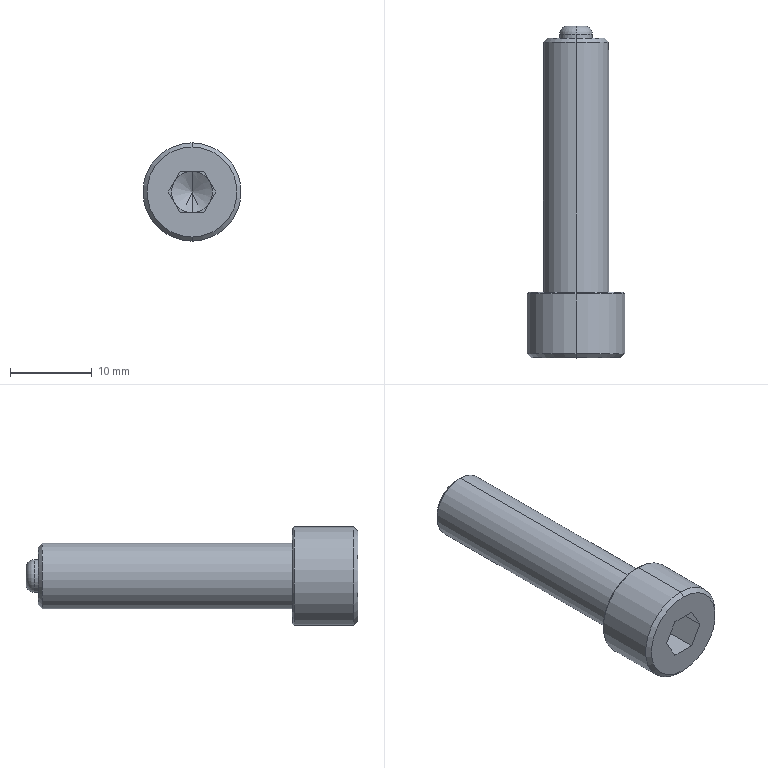Part | SolidWorks | features ICE 4, Chamfer 2, CirPattern 1, Extrusion 1, Fillet 1, RevCut 1 | 1 solid | 32 faces | box 12 x 40.5 x 12 mm | volume 2375 mm3 | plane 16 | cone 8 | cylinder 6 | torus 2 | commonest cylinder face diameters 4 x2 8 x2 12 x2
STEP:
#1=CARTESIAN_POINT('',(0.,1.443,0.));
#2=VERTEX_POINT('',#1);
#3=CARTESIAN_POINT('',(0.,0.,-2.5));
#4=VERTEX_POINT('',#3);
#5=CARTESIAN_POINT('',(0.,0.,-2.5));
#6=DIRECTION('',(0.,-0.5,-0.866));
#7=VECTOR('',#6,1000.);
#8=LINE('',#5,#7);
#9=EDGE_CURVE('',#2,#4,#8,.T.);
#10=ORIENTED_EDGE('',*,*,#9,.F.);
#11=CARTESIAN_POINT('',(0.,0.,2.5));
#12=VERTEX_POINT('',#11);
#13=CARTESIAN_POINT('',(0.,0.,2.5));
#14=DIRECTION('',(0.,-0.5,0.866));
#15=VECTOR('',#14,1000.);
#16=LINE('',#13,#15);
#17=EDGE_CURVE('',#2,#12,#16,.T.);
#18=ORIENTED_EDGE('',*,*,#17,.T.);
#19=CARTESIAN_POINT('',(-2.165,0.,1.25));
#20=VERTEX_POINT('',#19);
#21=CARTESIAN_POINT('',(0.,0.,0.));
#22=DIRECTION('',(0.,1.,0.));
#23=DIRECTION('',(0.,0.,-1.));
#24=AXIS2_PLACEMENT_3D('',#21,#22,#23);
#25=CIRCLE('',#24,2.5);
#26=EDGE_CURVE('',#20,#12,#25,.T.);
#27=ORIENTED_EDGE('',*,*,#26,.F.);
#28=CARTESIAN_POINT('',(-2.165,0.,-1.25));
#29=VERTEX_POINT('',#28);
#30=CARTESIAN_POINT('',(0.,0.,0.));
#31=DIRECTION('',(0.,1.,0.));
#32=DIRECTION('',(0.,0.,-1.));
#33=AXIS2_PLACEMENT_3D('',#30,#31,#32);
#34=CIRCLE('',#33,2.5);
#35=EDGE_CURVE('',#29,#20,#34,.T.);
#36=ORIENTED_EDGE('',*,*,#35,.F.);
#37=CARTESIAN_POINT('',(0.,0.,0.));
#38=DIRECTION('',(0.,1.,0.));
#39=DIRECTION('',(0.,0.,-1.));
#40=AXIS2_PLACEMENT_3D('',#37,#38,#39);
#41=CIRCLE('',#40,2.5);
#42=EDGE_CURVE('',#4,#29,#41,.T.);
#43=ORIENTED_EDGE('',*,*,#42,.F.);
#44=EDGE_LOOP('',(#10,#18,#27,#36,#43));
#45=FACE_OUTER_BOUND('',#44,.T.);
#46=CARTESIAN_POINT('',(0.,0.,0.));
#47=DIRECTION('',(0.,-1.,0.));
#48=DIRECTION('',(0.,0.,-1.));
#49=AXIS2_PLACEMENT_3D('',#46,#47,#48);
#50=CONICAL_SURFACE('',#49,2.5,1.047);
#51=ADVANCED_FACE('',(#45),#50,.F.);
#52=CARTESIAN_POINT('',(0.,35.5,-2.));
#53=VERTEX_POINT('',#52);
#54=CARTESIAN_POINT('',(0.,35.5,2.));
#55=VERTEX_POINT('',#54);
#56=CARTESIAN_POINT('',(0.,35.5,0.));
#57=DIRECTION('',(0.,-1.,0.));
#58=DIRECTION('',(0.,0.,1.));
#59=AXIS2_PLACEMENT_3D('',#56,#57,#58);
#60=CIRCLE('',#59,2.);
#61=EDGE_CURVE('',#53,#55,#60,.T.);
#62=ORIENTED_EDGE('',*,*,#61,.F.);
#63=CARTESIAN_POINT('',(0.,36.5,-1.));
#64=VERTEX_POINT('',#63);
#65=CARTESIAN_POINT('',(0.,35.5,-1.));
#66=DIRECTION('',(1.,0.,0.));
#67=DIRECTION('',(0.,0.,-1.));
#68=AXIS2_PLACEMENT_3D('',#65,#66,#67);
#69=CIRCLE('',#68,1.);
#70=EDGE_CURVE('',#53,#64,#69,.T.);
#71=ORIENTED_EDGE('',*,*,#70,.T.);
#72=CARTESIAN_POINT('',(0.,36.5,1.));
#73=VERTEX_POINT('',#72);
#74=CARTESIAN_POINT('',(0.,36.5,0.));
#75=DIRECTION('',(0.,1.,0.));
#76=DIRECTION('',(0.,0.,1.));
#77=AXIS2_PLACEMENT_3D('',#74,#75,#76);
#78=CIRCLE('',#77,1.);
#79=EDGE_CURVE('',#73,#64,#78,.T.);
#80=ORIENTED_EDGE('',*,*,#79,.F.);
#81=CARTESIAN_POINT('',(0.,35.5,1.));
#82=DIRECTION('',(-1.,0.,0.));
#83=DIRECTION('',(0.,0.,1.));
#84=AXIS2_PLACEMENT_3D('',#81,#82,#83);
#85=CIRCLE('',#84,1.);
#86=EDGE_CURVE('',#55,#73,#85,.T.);
#87=ORIENTED_EDGE('',*,*,#86,.F.);
#88=EDGE_LOOP('',(#62,#71,#80,#87));
#89=FACE_OUTER_BOUND('',#88,.T.);
#90=CARTESIAN_POINT('',(0.,35.5,0.));
#91=DIRECTION('',(0.,1.,0.));
#92=DIRECTION('',(0.,0.,1.));
#93=AXIS2_PLACEMENT_3D('',#90,#91,#92);
#94=TOROIDAL_SURFACE('',#93,1.,1.);
#95=ADVANCED_FACE('',(#89),#94,.T.);
#96=CARTESIAN_POINT('',(0.,4.,5.8));
#97=VERTEX_POINT('',#96);
#98=CARTESIAN_POINT('',(0.,4.,-5.8));
#99=VERTEX_POINT('',#98);
#100=CARTESIAN_POINT('',(0.,4.,0.));
#101=DIRECTION('',(0.,1.,0.));
#102=DIRECTION('',(0.,0.,1.));
#103=AXIS2_PLACEMENT_3D('',#100,#101,#102);
#104=CIRCLE('',#103,5.8);
#105=EDGE_CURVE('',#97,#99,#104,.T.);
#106=ORIENTED_EDGE('',*,*,#105,.F.);
#107=CARTESIAN_POINT('',(0.,3.8,6.));
#108=VERTEX_POINT('',#107);
#109=CARTESIAN_POINT('',(0.,4.,5.8));
#110=DIRECTION('',(0.,-0.7071,0.7071));
#111=VECTOR('',#110,1000.);
#112=LINE('',#109,#111);
#113=EDGE_CURVE('',#97,#108,#112,.T.);
#114=ORIENTED_EDGE('',*,*,#113,.T.);
#115=CARTESIAN_POINT('',(0.,3.8,-6.));
#116=VERTEX_POINT('',#115);
#117=CARTESIAN_POINT('',(0.,3.8,0.));
#118=DIRECTION('',(0.,-1.,0.));
#119=DIRECTION('',(0.,0.,1.));
#120=AXIS2_PLACEMENT_3D('',#117,#118,#119);
#121=CIRCLE('',#120,6.);
#122=EDGE_CURVE('',#116,#108,#121,.T.);
#123=ORIENTED_EDGE('',*,*,#122,.F.);
#124=CARTESIAN_POINT('',(0.,4.,-5.8));
#125=DIRECTION('',(0.,-0.7071,-0.7071));
#126=VECTOR('',#125,1000.);
#127=LINE('',#124,#126);
#128=EDGE_CURVE('',#99,#116,#127,.T.);
#129=ORIENTED_EDGE('',*,*,#128,.F.);
#130=EDGE_LOOP('',(#106,#114,#123,#129));
#131=FACE_OUTER_BOUND('',#130,.T.);
#132=CARTESIAN_POINT('',(0.,4.,0.));
#133=DIRECTION('',(0.,-1.,0.));
#134=DIRECTION('',(0.,0.,-1.));
#135=AXIS2_PLACEMENT_3D('',#132,#133,#134);
#136=CONICAL_SURFACE('',#135,5.8,0.7854);
#137=ADVANCED_FACE('',(#131),#136,.T.);
#138=CARTESIAN_POINT('',(0.,-4.,-5.5));
#139=VERTEX_POINT('',#138);
#140=CARTESIAN_POINT('',(0.,-4.,5.5));
#141=VERTEX_POINT('',#140);
#142=CARTESIAN_POINT('',(0.,-4.,0.));
#143=DIRECTION('',(0.,-1.,0.));
#144=DIRECTION('',(0.,0.,1.));
#145=AXIS2_PLACEMENT_3D('',#142,#143,#144);
#146=CIRCLE('',#145,5.5);
#147=EDGE_CURVE('',#139,#141,#146,.T.);
#148=ORIENTED_EDGE('',*,*,#147,.F.);
#149=CARTESIAN_POINT('',(0.,-3.5,-6.));
#150=VERTEX_POINT('',#149);
#151=CARTESIAN_POINT('',(0.,-3.5,-6.));
#152=DIRECTION('',(0.,0.7071,-0.7071));
#153=VECTOR('',#152,1000.);
#154=LINE('',#151,#153);
#155=EDGE_CURVE('',#139,#150,#154,.T.);
#156=ORIENTED_EDGE('',*,*,#155,.T.);
#157=CARTESIAN_POINT('',(0.,-3.5,6.));
#158=VERTEX_POINT('',#157);
#159=CARTESIAN_POINT('',(0.,-3.5,0.));
#160=DIRECTION('',(0.,1.,0.));
#161=DIRECTION('',(0.,0.,1.));
#162=AXIS2_PLACEMENT_3D('',#159,#160,#161);
#163=CIRCLE('',#162,6.);
#164=EDGE_CURVE('',#158,#150,#163,.T.);
#165=ORIENTED_EDGE('',*,*,#164,.F.);
#166=CARTESIAN_POINT('',(0.,-3.5,6.));
#167=DIRECTION('',(0.,0.7071,0.7071));
#168=VECTOR('',#167,1000.);
#169=LINE('',#166,#168);
#170=EDGE_CURVE('',#141,#158,#169,.T.);
#171=ORIENTED_EDGE('',*,*,#170,.F.);
#172=EDGE_LOOP('',(#148,#156,#165,#171));
#173=FACE_OUTER_BOUND('',#172,.T.);
#174=CARTESIAN_POINT('',(0.,-3.5,0.));
#175=DIRECTION('',(0.,1.,0.));
#176=DIRECTION('',(0.,0.,1.));
#177=AXIS2_PLACEMENT_3D('',#174,#175,#176);
#178=CONICAL_SURFACE('',#177,6.,0.7854);
#179=ADVANCED_FACE('',(#173),#178,.T.);
#180=CARTESIAN_POINT('',(0.,35.,3.5));
#181=VERTEX_POINT('',#180);
#182=CARTESIAN_POINT('',(0.,35.,-3.5));
#183=VERTEX_POINT('',#182);
#184=CARTESIAN_POINT('',(0.,35.,0.));
#185=DIRECTION('',(0.,1.,0.));
#186=DIRECTION('',(0.,0.,1.));
#187=AXIS2_PLACEMENT_3D('',#184,#185,#186);
#188=CIRCLE('',#187,3.5);
#189=EDGE_CURVE('',#181,#183,#188,.T.);
#190=ORIENTED_EDGE('',*,*,#189,.F.);
#191=CARTESIAN_POINT('',(0.,34.5,4.));
#192=VERTEX_POINT('',#191);
#193=CARTESIAN_POINT('',(0.,35.,3.5));
#194=DIRECTION('',(0.,-0.7071,0.7071));
#195=VECTOR('',#194,1000.);
#196=LINE('',#193,#195);
#197=EDGE_CURVE('',#181,#192,#196,.T.);
#198=ORIENTED_EDGE('',*,*,#197,.T.);
#199=CARTESIAN_POINT('',(0.,34.5,-4.));
#200=VERTEX_POINT('',#199);
#201=CARTESIAN_POINT('',(0.,34.5,0.));
#202=DIRECTION('',(0.,-1.,0.));
#203=DIRECTION('',(0.,0.,1.));
#204=AXIS2_PLACEMENT_3D('',#201,#202,#203);
#205=CIRCLE('',#204,4.);
#206=EDGE_CURVE('',#200,#192,#205,.T.);
#207=ORIENTED_EDGE('',*,*,#206,.F.);
#208=CARTESIAN_POINT('',(0.,35.,-3.5));
#209=DIRECTION('',(0.,-0.7071,-0.7071));
#210=VECTOR('',#209,1000.);
#211=LINE('',#208,#210);
#212=EDGE_CURVE('',#183,#200,#211,.T.);
#213=ORIENTED_EDGE('',*,*,#212,.F.);
#214=EDGE_LOOP('',(#190,#198,#207,#213));
#215=FACE_OUTER_BOUND('',#214,.T.);
#216=CARTESIAN_POINT('',(0.,35.,0.));
#217=DIRECTION('',(0.,-1.,0.));
#218=DIRECTION('',(0.,0.,-1.));
#219=AXIS2_PLACEMENT_3D('',#216,#217,#218);
#220=CONICAL_SURFACE('',#219,3.5,0.7854);
#221=ADVANCED_FACE('',(#215),#220,.T.);
#222=ORIENTED_EDGE('',*,*,#61,.T.);
#223=CARTESIAN_POINT('',(0.,35.,2.));
#224=VERTEX_POINT('',#223);
#225=CARTESIAN_POINT('',(0.,36.5,2.));
#226=DIRECTION('',(0.,-1.,0.));
#227=VECTOR('',#226,1000.);
#228=LINE('',#225,#227);
#229=EDGE_CURVE('',#55,#224,#228,.T.);
#230=ORIENTED_EDGE('',*,*,#229,.T.);
#231=CARTESIAN_POINT('',(0.,35.,-2.));
#232=VERTEX_POINT('',#231);
#233=CARTESIAN_POINT('',(0.,35.,0.));
#234=DIRECTION('',(0.,1.,0.));
#235=DIRECTION('',(0.,0.,1.));
#236=AXIS2_PLACEMENT_3D('',#233,#234,#235);
#237=CIRCLE('',#236,2.);
#238=EDGE_CURVE('',#224,#232,#237,.T.);
#239=ORIENTED_EDGE('',*,*,#238,.T.);
#240=CARTESIAN_POINT('',(0.,36.5,-2.));
#241=DIRECTION('',(0.,-1.,0.));
#242=VECTOR('',#241,1000.);
#243=LINE('',#240,#242);
#244=EDGE_CURVE('',#53,#232,#243,.T.);
#245=ORIENTED_EDGE('',*,*,#244,.F.);
#246=EDGE_LOOP('',(#222,#230,#239,#245));
#247=FACE_OUTER_BOUND('',#246,.T.);
#248=CARTESIAN_POINT('',(0.,36.5,0.));
#249=DIRECTION('',(0.,-1.,0.));
#250=DIRECTION('',(0.,0.,-1.));
#251=AXIS2_PLACEMENT_3D('',#248,#249,#250);
#252=CYLINDRICAL_SURFACE('',#251,2.);
#253=ADVANCED_FACE('',(#247),#252,.T.);
#254=ORIENTED_EDGE('',*,*,#206,.T.);
#255=CARTESIAN_POINT('',(0.,4.,4.));
#256=VERTEX_POINT('',#255);
#257=CARTESIAN_POINT('',(0.,35.,4.));
#258=DIRECTION('',(0.,-1.,0.));
#259=VECTOR('',#258,1000.);
#260=LINE('',#257,#259);
#261=EDGE_CURVE('',#192,#256,#260,.T.);
#262=ORIENTED_EDGE('',*,*,#261,.T.);
#263=CARTESIAN_POINT('',(0.,4.,-4.));
#264=VERTEX_POINT('',#263);
#265=CARTESIAN_POINT('',(0.,4.,0.));
#266=DIRECTION('',(0.,1.,0.));
#267=DIRECTION('',(0.,0.,1.));
#268=AXIS2_PLACEMENT_3D('',#265,#266,#267);
#269=CIRCLE('',#268,4.);
#270=EDGE_CURVE('',#256,#264,#269,.T.);
#271=ORIENTED_EDGE('',*,*,#270,.T.);
#272=CARTESIAN_POINT('',(0.,35.,-4.));
#273=DIRECTION('',(0.,-1.,0.));
#274=VECTOR('',#273,1000.);
#275=LINE('',#272,#274);
#276=EDGE_CURVE('',#200,#264,#275,.T.);
#277=ORIENTED_EDGE('',*,*,#276,.F.);
#278=EDGE_LOOP('',(#254,#262,#271,#277));
#279=FACE_OUTER_BOUND('',#278,.T.);
#280=CARTESIAN_POINT('',(0.,35.,0.));
#281=DIRECTION('',(0.,-1.,0.));
#282=DIRECTION('',(0.,0.,-1.));
#283=AXIS2_PLACEMENT_3D('',#280,#281,#282);
#284=CYLINDRICAL_SURFACE('',#283,4.);
#285=ADVANCED_FACE('',(#279),#284,.T.);
#286=ORIENTED_EDGE('',*,*,#122,.T.);
#287=CARTESIAN_POINT('',(0.,4.,6.));
#288=DIRECTION('',(0.,-1.,0.));
#289=VECTOR('',#288,1000.);
#290=LINE('',#287,#289);
#291=EDGE_CURVE('',#108,#158,#290,.T.);
#292=ORIENTED_EDGE('',*,*,#291,.T.);
#293=ORIENTED_EDGE('',*,*,#164,.T.);
#294=CARTESIAN_POINT('',(0.,4.,-6.));
#295=DIRECTION('',(0.,-1.,0.));
#296=VECTOR('',#295,1000.);
#297=LINE('',#294,#296);
#298=EDGE_CURVE('',#116,#150,#297,.T.);
#299=ORIENTED_EDGE('',*,*,#298,.F.);
#300=EDGE_LOOP('',(#286,#292,#293,#299));
#301=FACE_OUTER_BOUND('',#300,.T.);
#302=CARTESIAN_POINT('',(0.,4.,0.));
#303=DIRECTION('',(0.,-1.,0.));
#304=DIRECTION('',(0.,0.,-1.));
#305=AXIS2_PLACEMENT_3D('',#302,#303,#304);
#306=CYLINDRICAL_SURFACE('',#305,6.);
#307=ADVANCED_FACE('',(#301),#306,.T.);
#308=CARTESIAN_POINT('',(-1.443,0.,-2.5));
#309=VERTEX_POINT('',#308);
#310=CARTESIAN_POINT('',(-1.443,0.,-2.5));
#311=DIRECTION('',(1.,0.,0.));
#312=VECTOR('',#311,1000.);
#313=LINE('',#310,#312);
#314=EDGE_CURVE('',#309,#4,#313,.T.);
#315=ORIENTED_EDGE('',*,*,#314,.T.);
#316=ORIENTED_EDGE('',*,*,#42,.T.);
#317=CARTESIAN_POINT('',(-2.887,0.,0.));
#318=DIRECTION('',(0.5,0.,-0.866));
#319=VECTOR('',#318,1000.);
#320=LINE('',#317,#319);
#321=EDGE_CURVE('',#29,#309,#320,.T.);
#322=ORIENTED_EDGE('',*,*,#321,.T.);
#323=EDGE_LOOP('',(#315,#316,#322));
#324=FACE_OUTER_BOUND('',#323,.T.);
#325=CARTESIAN_POINT('',(0.,0.,0.));
#326=DIRECTION('',(0.,-1.,0.));
#327=DIRECTION('',(0.,0.,-1.));
#328=AXIS2_PLACEMENT_3D('',#325,#326,#327);
#329=PLANE('',#328);
#330=ADVANCED_FACE('',(#324),#329,.T.);
#331=CARTESIAN_POINT('',(-2.887,0.,0.));
#332=VERTEX_POINT('',#331);
#333=CARTESIAN_POINT('',(-2.887,0.,0.));
#334=DIRECTION('',(0.5,0.,-0.866));
#335=VECTOR('',#334,1000.);
#336=LINE('',#333,#335);
#337=EDGE_CURVE('',#332,#29,#336,.T.);
#338=ORIENTED_EDGE('',*,*,#337,.T.);
#339=ORIENTED_EDGE('',*,*,#35,.T.);
#340=CARTESIAN_POINT('',(-1.443,0.,2.5));
#341=DIRECTION('',(-0.5,0.,-0.866));
#342=VECTOR('',#341,1000.);
#343=LINE('',#340,#342);
#344=EDGE_CURVE('',#20,#332,#343,.T.);
#345=ORIENTED_EDGE('',*,*,#344,.T.);
#346=EDGE_LOOP('',(#338,#339,#345));
#347=FACE_OUTER_BOUND('',#346,.T.);
#348=CARTESIAN_POINT('',(0.,0.,0.));
#349=DIRECTION('',(0.,-1.,0.));
#350=DIRECTION('',(0.,0.,-1.));
#351=AXIS2_PLACEMENT_3D('',#348,#349,#350);
#352=PLANE('',#351);
#353=ADVANCED_FACE('',(#347),#352,.T.);
#354=CARTESIAN_POINT('',(-1.443,0.,2.5));
#355=VERTEX_POINT('',#354);
#356=CARTESIAN_POINT('',(-1.443,0.,2.5));
#357=DIRECTION('',(-0.5,0.,-0.866));
#358=VECTOR('',#357,1000.);
#359=LINE('',#356,#358);
#360=EDGE_CURVE('',#355,#20,#359,.T.);
#361=ORIENTED_EDGE('',*,*,#360,.T.);
#362=ORIENTED_EDGE('',*,*,#26,.T.);
#363=CARTESIAN_POINT('',(1.443,0.,2.5));
#364=DIRECTION('',(-1.,0.,0.));
#365=VECTOR('',#364,1000.);
#366=LINE('',#363,#365);
#367=EDGE_CURVE('',#12,#355,#366,.T.);
#368=ORIENTED_EDGE('',*,*,#367,.T.);
#369=EDGE_LOOP('',(#361,#362,#368));
#370=FACE_OUTER_BOUND('',#369,.T.);
#371=CARTESIAN_POINT('',(0.,0.,0.));
#372=DIRECTION('',(0.,-1.,0.));
#373=DIRECTION('',(0.,0.,-1.));
#374=AXIS2_PLACEMENT_3D('',#371,#372,#373);
#375=PLANE('',#374);
#376=ADVANCED_FACE('',(#370),#375,.T.);
#377=CARTESIAN_POINT('',(1.443,0.,2.5));
#378=VERTEX_POINT('',#377);
#379=CARTESIAN_POINT('',(1.443,0.,2.5));
#380=DIRECTION('',(-1.,0.,0.));
#381=VECTOR('',#380,1000.);
#382=LINE('',#379,#381);
#383=EDGE_CURVE('',#378,#12,#382,.T.);
#384=ORIENTED_EDGE('',*,*,#383,.T.);
#385=CARTESIAN_POINT('',(2.165,0.,1.25));
#386=VERTEX_POINT('',#385);
#387=CARTESIAN_POINT('',(0.,0.,0.));
#388=DIRECTION('',(0.,1.,0.));
#389=DIRECTION('',(0.,0.,1.));
#390=AXIS2_PLACEMENT_3D('',#387,#388,#389);
#391=CIRCLE('',#390,2.5);
#392=EDGE_CURVE('',#12,#386,#391,.T.);
#393=ORIENTED_EDGE('',*,*,#392,.T.);
#394=CARTESIAN_POINT('',(2.887,0.,0.));
#395=DIRECTION('',(-0.5,0.,0.866));
#396=VECTOR('',#395,1000.);
#397=LINE('',#394,#396);
#398=EDGE_CURVE('',#386,#378,#397,.T.);
#399=ORIENTED_EDGE('',*,*,#398,.T.);
#400=EDGE_LOOP('',(#384,#393,#399));
#401=FACE_OUTER_BOUND('',#400,.T.);
#402=CARTESIAN_POINT('',(0.,0.,0.));
#403=DIRECTION('',(0.,-1.,0.));
#404=DIRECTION('',(0.,0.,-1.));
#405=AXIS2_PLACEMENT_3D('',#402,#403,#404);
#406=PLANE('',#405);
#407=ADVANCED_FACE('',(#401),#406,.T.);
#408=CARTESIAN_POINT('',(2.887,0.,0.));
#409=VERTEX_POINT('',#408);
#410=CARTESIAN_POINT('',(2.887,0.,0.));
#411=DIRECTION('',(-0.5,0.,0.866));
#412=VECTOR('',#411,1000.);
#413=LINE('',#410,#412);
#414=EDGE_CURVE('',#409,#386,#413,.T.);
#415=ORIENTED_EDGE('',*,*,#414,.T.);
#416=CARTESIAN_POINT('',(2.165,0.,-1.25));
#417=VERTEX_POINT('',#416);
#418=CARTESIAN_POINT('',(0.,0.,0.));
#419=DIRECTION('',(0.,1.,0.));
#420=DIRECTION('',(0.,0.,-1.));
#421=AXIS2_PLACEMENT_3D('',#418,#419,#420);
#422=CIRCLE('',#421,2.5);
#423=EDGE_CURVE('',#386,#417,#422,.T.);
#424=ORIENTED_EDGE('',*,*,#423,.T.);
#425=CARTESIAN_POINT('',(1.443,0.,-2.5));
#426=DIRECTION('',(0.5,0.,0.866));
#427=VECTOR('',#426,1000.);
#428=LINE('',#425,#427);
#429=EDGE_CURVE('',#417,#409,#428,.T.);
#430=ORIENTED_EDGE('',*,*,#429,.T.);
#431=EDGE_LOOP('',(#415,#424,#430));
#432=FACE_OUTER_BOUND('',#431,.T.);
#433=CARTESIAN_POINT('',(0.,0.,0.));
#434=DIRECTION('',(0.,-1.,0.));
#435=DIRECTION('',(0.,0.,-1.));
#436=AXIS2_PLACEMENT_3D('',#433,#434,#435);
#437=PLANE('',#436);
#438=ADVANCED_FACE('',(#432),#437,.T.);
#439=CARTESIAN_POINT('',(1.443,0.,-2.5));
#440=VERTEX_POINT('',#439);
#441=CARTESIAN_POINT('',(1.443,0.,-2.5));
#442=DIRECTION('',(0.5,0.,0.866));
#443=VECTOR('',#442,1000.);
#444=LINE('',#441,#443);
#445=EDGE_CURVE('',#440,#417,#444,.T.);
#446=ORIENTED_EDGE('',*,*,#445,.T.);
#447=CARTESIAN_POINT('',(0.,0.,0.));
#448=DIRECTION('',(0.,1.,0.));
#449=DIRECTION('',(0.,0.,-1.));
#450=AXIS2_PLACEMENT_3D('',#447,#448,#449);
#451=CIRCLE('',#450,2.5);
#452=EDGE_CURVE('',#417,#4,#451,.T.);
#453=ORIENTED_EDGE('',*,*,#452,.T.);
#454=CARTESIAN_POINT('',(-1.443,0.,-2.5));
#455=DIRECTION('',(1.,0.,0.));
#456=VECTOR('',#455,1000.);
#457=LINE('',#454,#456);
#458=EDGE_CURVE('',#4,#440,#457,.T.);
#459=ORIENTED_EDGE('',*,*,#458,.T.);
#460=EDGE_LOOP('',(#446,#453,#459));
#461=FACE_OUTER_BOUND('',#460,.T.);
#462=CARTESIAN_POINT('',(0.,0.,0.));
#463=DIRECTION('',(0.,-1.,0.));
#464=DIRECTION('',(0.,0.,-1.));
#465=AXIS2_PLACEMENT_3D('',#462,#463,#464);
#466=PLANE('',#465);
#467=ADVANCED_FACE('',(#461),#466,.T.);
#468=CARTESIAN_POINT('',(0.,35.,0.));
#469=DIRECTION('',(0.,1.,0.));
#470=DIRECTION('',(0.,0.,1.));
#471=AXIS2_PLACEMENT_3D('',#468,#469,#470);
#472=CIRCLE('',#471,3.5);
#473=EDGE_CURVE('',#183,#181,#472,.T.);
#474=ORIENTED_EDGE('',*,*,#473,.T.);
#475=ORIENTED_EDGE('',*,*,#189,.T.);
#476=EDGE_LOOP('',(#474,#475));
#477=FACE_OUTER_BOUND('',#476,.T.);
#478=CARTESIAN_POINT('',(0.,35.,0.));
#479=DIRECTION('',(0.,1.,0.));
#480=DIRECTION('',(0.,0.,1.));
#481=AXIS2_PLACEMENT_3D('',#478,#479,#480);
#482=CIRCLE('',#481,2.);
#483=EDGE_CURVE('',#232,#224,#482,.T.);
#484=ORIENTED_EDGE('',*,*,#483,.F.);
#485=ORIENTED_EDGE('',*,*,#238,.F.);
#486=EDGE_LOOP('',(#484,#485));
#487=FACE_BOUND('',#486,.T.);
#488=CARTESIAN_POINT('',(0.,35.,0.));
#489=DIRECTION('',(0.,1.,0.));
#490=DIRECTION('',(0.,0.,1.));
#491=AXIS2_PLACEMENT_3D('',#488,#489,#490);
#492=PLANE('',#491);
#493=ADVANCED_FACE('',(#477,#487),#492,.T.);
#494=CARTESIAN_POINT('',(0.,4.,0.));
#495=DIRECTION('',(0.,1.,0.));
#496=DIRECTION('',(0.,0.,1.));
#497=AXIS2_PLACEMENT_3D('',#494,#495,#496);
#498=CIRCLE('',#497,5.8);
#499=EDGE_CURVE('',#99,#97,#498,.T.);
#500=ORIENTED_EDGE('',*,*,#499,.T.);
#501=ORIENTED_EDGE('',*,*,#105,.T.);
#502=EDGE_LOOP('',(#500,#501));
#503=FACE_OUTER_BOUND('',#502,.T.);
#504=CARTESIAN_POINT('',(0.,4.,0.));
#505=DIRECTION('',(0.,1.,0.));
#506=DIRECTION('',(0.,0.,1.));
#507=AXIS2_PLACEMENT_3D('',#504,#505,#506);
#508=CIRCLE('',#507,4.);
#509=EDGE_CURVE('',#264,#256,#508,.T.);
#510=ORIENTED_EDGE('',*,*,#509,.F.);
#511=ORIENTED_EDGE('',*,*,#270,.F.);
#512=EDGE_LOOP('',(#510,#511));
#513=FACE_BOUND('',#512,.T.);
#514=CARTESIAN_POINT('',(0.,4.,0.));
#515=DIRECTION('',(0.,1.,0.));
#516=DIRECTION('',(0.,0.,1.));
#517=AXIS2_PLACEMENT_3D('',#514,#515,#516);
#518=PLANE('',#517);
#519=ADVANCED_FACE('',(#503,#513),#518,.T.);
#520=ORIENTED_EDGE('',*,*,#291,.F.);
#521=CARTESIAN_POINT('',(0.,3.8,0.));
#522=DIRECTION('',(0.,-1.,0.));
#523=DIRECTION('',(0.,0.,1.));
#524=AXIS2_PLACEMENT_3D('',#521,#522,#523);
#525=CIRCLE('',#524,6.);
#526=EDGE_CURVE('',#108,#116,#525,.T.);
#527=ORIENTED_EDGE('',*,*,#526,.T.);
#528=ORIENTED_EDGE('',*,*,#298,.T.);
#529=CARTESIAN_POINT('',(0.,-3.5,0.));
#530=DIRECTION('',(0.,1.,0.));
#531=DIRECTION('',(0.,0.,1.));
#532=AXIS2_PLACEMENT_3D('',#529,#530,#531);
#533=CIRCLE('',#532,6.);
#534=EDGE_CURVE('',#150,#158,#533,.T.);
#535=ORIENTED_EDGE('',*,*,#534,.T.);
#536=EDGE_LOOP('',(#520,#527,#528,#535));
#537=FACE_OUTER_BOUND('',#536,.T.);
#538=CARTESIAN_POINT('',(0.,4.,0.));
#539=DIRECTION('',(0.,-1.,0.));
#540=DIRECTION('',(0.,0.,-1.));
#541=AXIS2_PLACEMENT_3D('',#538,#539,#540);
#542=CYLINDRICAL_SURFACE('',#541,6.);
#543=ADVANCED_FACE('',(#537),#542,.T.);
#544=CARTESIAN_POINT('',(0.,-4.,0.));
#545=DIRECTION('',(0.,-1.,0.));
#546=DIRECTION('',(0.,0.,1.));
#547=AXIS2_PLACEMENT_3D('',#544,#545,#546);
#548=CIRCLE('',#547,5.5);
#549=EDGE_CURVE('',#141,#139,#548,.T.);
#550=ORIENTED_EDGE('',*,*,#549,.T.);
#551=ORIENTED_EDGE('',*,*,#147,.T.);
#552=EDGE_LOOP('',(#550,#551));
#553=FACE_OUTER_BOUND('',#552,.T.);
#554=CARTESIAN_POINT('',(2.887,-4.,0.));
#555=VERTEX_POINT('',#554);
#556=CARTESIAN_POINT('',(1.443,-4.,2.5));
#557=VERTEX_POINT('',#556);
#558=CARTESIAN_POINT('',(2.887,-4.,0.));
#559=DIRECTION('',(-0.5,0.,0.866));
#560=VECTOR('',#559,1000.);
#561=LINE('',#558,#560);
#562=EDGE_CURVE('',#555,#557,#561,.T.);
#563=ORIENTED_EDGE('',*,*,#562,.F.);
#564=CARTESIAN_POINT('',(1.443,-4.,-2.5));
#565=VERTEX_POINT('',#564);
#566=CARTESIAN_POINT('',(1.443,-4.,-2.5));
#567=DIRECTION('',(0.5,0.,0.866));
#568=VECTOR('',#567,1000.);
#569=LINE('',#566,#568);
#570=EDGE_CURVE('',#565,#555,#569,.T.);
#571=ORIENTED_EDGE('',*,*,#570,.F.);
#572=CARTESIAN_POINT('',(-1.443,-4.,-2.5));
#573=VERTEX_POINT('',#572);
#574=CARTESIAN_POINT('',(-1.443,-4.,-2.5));
#575=DIRECTION('',(1.,0.,0.));
#576=VECTOR('',#575,1000.);
#577=LINE('',#574,#576);
#578=EDGE_CURVE('',#573,#565,#577,.T.);
#579=ORIENTED_EDGE('',*,*,#578,.F.);
#580=CARTESIAN_POINT('',(-2.887,-4.,0.));
#581=VERTEX_POINT('',#580);
#582=CARTESIAN_POINT('',(-2.887,-4.,0.));
#583=DIRECTION('',(0.5,0.,-0.866));
#584=VECTOR('',#583,1000.);
#585=LINE('',#582,#584);
#586=EDGE_CURVE('',#581,#573,#585,.T.);
#587=ORIENTED_EDGE('',*,*,#586,.F.);
#588=CARTESIAN_POINT('',(-1.443,-4.,2.5));
#589=VERTEX_POINT('',#588);
#590=CARTESIAN_POINT('',(-1.443,-4.,2.5));
#591=DIRECTION('',(-0.5,0.,-0.866));
#592=VECTOR('',#591,1000.);
#593=LINE('',#590,#592);
#594=EDGE_CURVE('',#589,#581,#593,.T.);
#595=ORIENTED_EDGE('',*,*,#594,.F.);
#596=CARTESIAN_POINT('',(1.443,-4.,2.5));
#597=DIRECTION('',(-1.,0.,0.));
#598=VECTOR('',#597,1000.);
#599=LINE('',#596,#598);
#600=EDGE_CURVE('',#557,#589,#599,.T.);
#601=ORIENTED_EDGE('',*,*,#600,.F.);
#602=EDGE_LOOP('',(#563,#571,#579,#587,#595,#601));
#603=FACE_BOUND('',#602,.T.);
#604=CARTESIAN_POINT('',(0.,-4.,0.));
#605=DIRECTION('',(0.,1.,0.));
#606=DIRECTION('',(0.,0.,1.));
#607=AXIS2_PLACEMENT_3D('',#604,#605,#606);
#608=PLANE('',#607);
#609=ADVANCED_FACE('',(#553,#603),#608,.F.);
#610=ORIENTED_EDGE('',*,*,#261,.F.);
#611=CARTESIAN_POINT('',(0.,34.5,0.));
#612=DIRECTION('',(0.,-1.,0.));
#613=DIRECTION('',(0.,0.,1.));
#614=AXIS2_PLACEMENT_3D('',#611,#612,#613);
#615=CIRCLE('',#614,4.);
#616=EDGE_CURVE('',#192,#200,#615,.T.);
#617=ORIENTED_EDGE('',*,*,#616,.T.);
#618=ORIENTED_EDGE('',*,*,#276,.T.);
#619=ORIENTED_EDGE('',*,*,#509,.T.);
#620=EDGE_LOOP('',(#610,#617,#618,#619));
#621=FACE_OUTER_BOUND('',#620,.T.);
#622=CARTESIAN_POINT('',(0.,35.,0.));
#623=DIRECTION('',(0.,-1.,0.));
#624=DIRECTION('',(0.,0.,-1.));
#625=AXIS2_PLACEMENT_3D('',#622,#623,#624);
#626=CYLINDRICAL_SURFACE('',#625,4.);
#627=ADVANCED_FACE('',(#621),#626,.T.);
#628=ORIENTED_EDGE('',*,*,#229,.F.);
#629=CARTESIAN_POINT('',(0.,35.5,0.));
#630=DIRECTION('',(0.,-1.,0.));
#631=DIRECTION('',(0.,0.,1.));
#632=AXIS2_PLACEMENT_3D('',#629,#630,#631);
#633=CIRCLE('',#632,2.);
#634=EDGE_CURVE('',#55,#53,#633,.T.);
#635=ORIENTED_EDGE('',*,*,#634,.T.);
#636=ORIENTED_EDGE('',*,*,#244,.T.);
#637=ORIENTED_EDGE('',*,*,#483,.T.);
#638=EDGE_LOOP('',(#628,#635,#636,#637));
#639=FACE_OUTER_BOUND('',#638,.T.);
#640=CARTESIAN_POINT('',(0.,36.5,0.));
#641=DIRECTION('',(0.,-1.,0.));
#642=DIRECTION('',(0.,0.,-1.));
#643=AXIS2_PLACEMENT_3D('',#640,#641,#642);
#644=CYLINDRICAL_SURFACE('',#643,2.);
#645=ADVANCED_FACE('',(#639),#644,.T.);
#646=ORIENTED_EDGE('',*,*,#79,.T.);
#647=CARTESIAN_POINT('',(0.,36.5,0.));
#648=DIRECTION('',(0.,1.,0.));
#649=DIRECTION('',(0.,0.,1.));
#650=AXIS2_PLACEMENT_3D('',#647,#648,#649);
#651=CIRCLE('',#650,1.);
#652=EDGE_CURVE('',#64,#73,#651,.T.);
#653=ORIENTED_EDGE('',*,*,#652,.T.);
#654=EDGE_LOOP('',(#646,#653));
#655=FACE_OUTER_BOUND('',#654,.T.);
#656=CARTESIAN_POINT('',(0.,36.5,0.));
#657=DIRECTION('',(0.,1.,0.));
#658=DIRECTION('',(0.,0.,1.));
#659=AXIS2_PLACEMENT_3D('',#656,#657,#658);
#660=PLANE('',#659);
#661=ADVANCED_FACE('',(#655),#660,.T.);
#662=ORIENTED_EDGE('',*,*,#570,.T.);
#663=CARTESIAN_POINT('',(2.887,0.,0.));
#664=DIRECTION('',(0.,-1.,0.));
#665=VECTOR('',#664,1000.);
#666=LINE('',#663,#665);
#667=EDGE_CURVE('',#409,#555,#666,.T.);
#668=ORIENTED_EDGE('',*,*,#667,.F.);
#669=ORIENTED_EDGE('',*,*,#429,.F.);
#670=ORIENTED_EDGE('',*,*,#445,.F.);
#671=CARTESIAN_POINT('',(1.443,0.,-2.5));
#672=DIRECTION('',(0.,-1.,0.));
#673=VECTOR('',#672,1000.);
#674=LINE('',#671,#673);
#675=EDGE_CURVE('',#440,#565,#674,.T.);
#676=ORIENTED_EDGE('',*,*,#675,.T.);
#677=EDGE_LOOP('',(#662,#668,#669,#670,#676));
#678=FACE_OUTER_BOUND('',#677,.T.);
#679=CARTESIAN_POINT('',(1.443,0.,-2.5));
#680=DIRECTION('',(0.866,0.,-0.5));
#681=DIRECTION('',(-0.5,0.,-0.866));
#682=AXIS2_PLACEMENT_3D('',#679,#680,#681);
#683=PLANE('',#682);
#684=ADVANCED_FACE('',(#678),#683,.F.);
#685=ORIENTED_EDGE('',*,*,#578,.T.);
#686=ORIENTED_EDGE('',*,*,#675,.F.);
#687=ORIENTED_EDGE('',*,*,#458,.F.);
#688=ORIENTED_EDGE('',*,*,#314,.F.);
#689=CARTESIAN_POINT('',(-1.443,0.,-2.5));
#690=DIRECTION('',(0.,-1.,0.));
#691=VECTOR('',#690,1000.);
#692=LINE('',#689,#691);
#693=EDGE_CURVE('',#309,#573,#692,.T.);
#694=ORIENTED_EDGE('',*,*,#693,.T.);
#695=EDGE_LOOP('',(#685,#686,#687,#688,#694));
#696=FACE_OUTER_BOUND('',#695,.T.);
#697=CARTESIAN_POINT('',(-1.443,0.,-2.5));
#698=DIRECTION('',(0.,0.,-1.));
#699=DIRECTION('',(-1.,0.,0.));
#700=AXIS2_PLACEMENT_3D('',#697,#698,#699);
#701=PLANE('',#700);
#702=ADVANCED_FACE('',(#696),#701,.F.);
#703=ORIENTED_EDGE('',*,*,#586,.T.);
#704=ORIENTED_EDGE('',*,*,#693,.F.);
#705=ORIENTED_EDGE('',*,*,#321,.F.);
#706=ORIENTED_EDGE('',*,*,#337,.F.);
#707=CARTESIAN_POINT('',(-2.887,0.,0.));
#708=DIRECTION('',(0.,-1.,0.));
#709=VECTOR('',#708,1000.);
#710=LINE('',#707,#709);
#711=EDGE_CURVE('',#332,#581,#710,.T.);
#712=ORIENTED_EDGE('',*,*,#711,.T.);
#713=EDGE_LOOP('',(#703,#704,#705,#706,#712));
#714=FACE_OUTER_BOUND('',#713,.T.);
#715=CARTESIAN_POINT('',(-2.887,0.,0.));
#716=DIRECTION('',(-0.866,0.,-0.5));
#717=DIRECTION('',(-0.5,0.,0.866));
#718=AXIS2_PLACEMENT_3D('',#715,#716,#717);
#719=PLANE('',#718);
#720=ADVANCED_FACE('',(#714),#719,.F.);
#721=ORIENTED_EDGE('',*,*,#594,.T.);
#722=ORIENTED_EDGE('',*,*,#711,.F.);
#723=ORIENTED_EDGE('',*,*,#344,.F.);
#724=ORIENTED_EDGE('',*,*,#360,.F.);
#725=CARTESIAN_POINT('',(-1.443,0.,2.5));
#726=DIRECTION('',(0.,-1.,0.));
#727=VECTOR('',#726,1000.);
#728=LINE('',#725,#727);
#729=EDGE_CURVE('',#355,#589,#728,.T.);
#730=ORIENTED_EDGE('',*,*,#729,.T.);
#731=EDGE_LOOP('',(#721,#722,#723,#724,#730));
#732=FACE_OUTER_BOUND('',#731,.T.);
#733=CARTESIAN_POINT('',(-1.443,0.,2.5));
#734=DIRECTION('',(-0.866,0.,0.5));
#735=DIRECTION('',(0.5,0.,0.866));
#736=AXIS2_PLACEMENT_3D('',#733,#734,#735);
#737=PLANE('',#736);
#738=ADVANCED_FACE('',(#732),#737,.F.);
#739=ORIENTED_EDGE('',*,*,#600,.T.);
#740=ORIENTED_EDGE('',*,*,#729,.F.);
#741=ORIENTED_EDGE('',*,*,#367,.F.);
#742=ORIENTED_EDGE('',*,*,#383,.F.);
#743=CARTESIAN_POINT('',(1.443,0.,2.5));
#744=DIRECTION('',(0.,-1.,0.));
#745=VECTOR('',#744,1000.);
#746=LINE('',#743,#745);
#747=EDGE_CURVE('',#378,#557,#746,.T.);
#748=ORIENTED_EDGE('',*,*,#747,.T.);
#749=EDGE_LOOP('',(#739,#740,#741,#742,#748));
#750=FACE_OUTER_BOUND('',#749,.T.);
#751=CARTESIAN_POINT('',(1.443,0.,2.5));
#752=DIRECTION('',(0.,0.,1.));
#753=DIRECTION('',(1.,0.,0.));
#754=AXIS2_PLACEMENT_3D('',#751,#752,#753);
#755=PLANE('',#754);
#756=ADVANCED_FACE('',(#750),#755,.F.);
#757=ORIENTED_EDGE('',*,*,#562,.T.);
#758=ORIENTED_EDGE('',*,*,#747,.F.);
#759=ORIENTED_EDGE('',*,*,#398,.F.);
#760=ORIENTED_EDGE('',*,*,#414,.F.);
#761=ORIENTED_EDGE('',*,*,#667,.T.);
#762=EDGE_LOOP('',(#757,#758,#759,#760,#761));
#763=FACE_OUTER_BOUND('',#762,.T.);
#764=CARTESIAN_POINT('',(2.887,0.,0.));
#765=DIRECTION('',(0.866,0.,0.5));
#766=DIRECTION('',(0.5,0.,-0.866));
#767=AXIS2_PLACEMENT_3D('',#764,#765,#766);
#768=PLANE('',#767);
#769=ADVANCED_FACE('',(#763),#768,.F.);
#770=ORIENTED_EDGE('',*,*,#197,.F.);
#771=ORIENTED_EDGE('',*,*,#473,.F.);
#772=ORIENTED_EDGE('',*,*,#212,.T.);
#773=ORIENTED_EDGE('',*,*,#616,.F.);
#774=EDGE_LOOP('',(#770,#771,#772,#773));
#775=FACE_OUTER_BOUND('',#774,.T.);
#776=CARTESIAN_POINT('',(0.,35.,0.));
#777=DIRECTION('',(0.,-1.,0.));
#778=DIRECTION('',(0.,0.,-1.));
#779=AXIS2_PLACEMENT_3D('',#776,#777,#778);
#780=CONICAL_SURFACE('',#779,3.5,0.7854);
#781=ADVANCED_FACE('',(#775),#780,.T.);
#782=ORIENTED_EDGE('',*,*,#155,.F.);
#783=ORIENTED_EDGE('',*,*,#549,.F.);
#784=ORIENTED_EDGE('',*,*,#170,.T.);
#785=ORIENTED_EDGE('',*,*,#534,.F.);
#786=EDGE_LOOP('',(#782,#783,#784,#785));
#787=FACE_OUTER_BOUND('',#786,.T.);
#788=CARTESIAN_POINT('',(0.,-3.5,0.));
#789=DIRECTION('',(0.,1.,0.));
#790=DIRECTION('',(0.,0.,1.));
#791=AXIS2_PLACEMENT_3D('',#788,#789,#790);
#792=CONICAL_SURFACE('',#791,6.,0.7854);
#793=ADVANCED_FACE('',(#787),#792,.T.);
#794=ORIENTED_EDGE('',*,*,#113,.F.);
#795=ORIENTED_EDGE('',*,*,#499,.F.);
#796=ORIENTED_EDGE('',*,*,#128,.T.);
#797=ORIENTED_EDGE('',*,*,#526,.F.);
#798=EDGE_LOOP('',(#794,#795,#796,#797));
#799=FACE_OUTER_BOUND('',#798,.T.);
#800=CARTESIAN_POINT('',(0.,4.,0.));
#801=DIRECTION('',(0.,-1.,0.));
#802=DIRECTION('',(0.,0.,-1.));
#803=AXIS2_PLACEMENT_3D('',#800,#801,#802);
#804=CONICAL_SURFACE('',#803,5.8,0.7854);
#805=ADVANCED_FACE('',(#799),#804,.T.);
#806=ORIENTED_EDGE('',*,*,#70,.F.);
#807=ORIENTED_EDGE('',*,*,#634,.F.);
#808=ORIENTED_EDGE('',*,*,#86,.T.);
#809=ORIENTED_EDGE('',*,*,#652,.F.);
#810=EDGE_LOOP('',(#806,#807,#808,#809));
#811=FACE_OUTER_BOUND('',#810,.T.);
#812=CARTESIAN_POINT('',(0.,35.5,0.));
#813=DIRECTION('',(0.,1.,0.));
#814=DIRECTION('',(0.,0.,1.));
#815=AXIS2_PLACEMENT_3D('',#812,#813,#814);
#816=TOROIDAL_SURFACE('',#815,1.,1.);
#817=ADVANCED_FACE('',(#811),#816,.T.);
#818=ORIENTED_EDGE('',*,*,#17,.F.);
#819=ORIENTED_EDGE('',*,*,#9,.T.);
#820=ORIENTED_EDGE('',*,*,#452,.F.);
#821=ORIENTED_EDGE('',*,*,#423,.F.);
#822=ORIENTED_EDGE('',*,*,#392,.F.);
#823=EDGE_LOOP('',(#818,#819,#820,#821,#822));
#824=FACE_OUTER_BOUND('',#823,.T.);
#825=CARTESIAN_POINT('',(0.,0.,0.));
#826=DIRECTION('',(0.,-1.,0.));
#827=DIRECTION('',(0.,0.,-1.));
#828=AXIS2_PLACEMENT_3D('',#825,#826,#827);
#829=CONICAL_SURFACE('',#828,2.5,1.047);
#830=ADVANCED_FACE('',(#824),#829,.F.);
#831=CLOSED_SHELL('',(#51,#95,#137,#179,#221,#253,#285,#307,#330,#353,#376,#407,#438,#467,#493,#519,#543,#609,#627,#645,#661,#684,#702,#720,#738,#756,#769,#781,#793,#805,#817,#830));
#832=MANIFOLD_SOLID_BREP('',#831);
#833=CARTESIAN_POINT('',(0.,0.,0.));
#834=DIRECTION('',(0.,0.,1.));
#835=DIRECTION('',(1.,0.,0.));
#836=AXIS2_PLACEMENT_3D('',#833,#834,#835);
#837=(LENGTH_UNIT()NAMED_UNIT(*)SI_UNIT(.MILLI.,.METRE.));
#838=UNCERTAINTY_MEASURE_WITH_UNIT(LENGTH_MEASURE(0.00001),#837,'','');
#839=(NAMED_UNIT(*)PLANE_ANGLE_UNIT()SI_UNIT($,.RADIAN.));
#840=(NAMED_UNIT(*)SI_UNIT($,.STERADIAN.)SOLID_ANGLE_UNIT());
#841=(GEOMETRIC_REPRESENTATION_CONTEXT(3)GLOBAL_UNCERTAINTY_ASSIGNED_CONTEXT((#838))GLOBAL_UNIT_ASSIGNED_CONTEXT((#837,#839,#840))REPRESENTATION_CONTEXT('',''));
#842=ADVANCED_BREP_SHAPE_REPRESENTATION('',(#832,#836),#841);